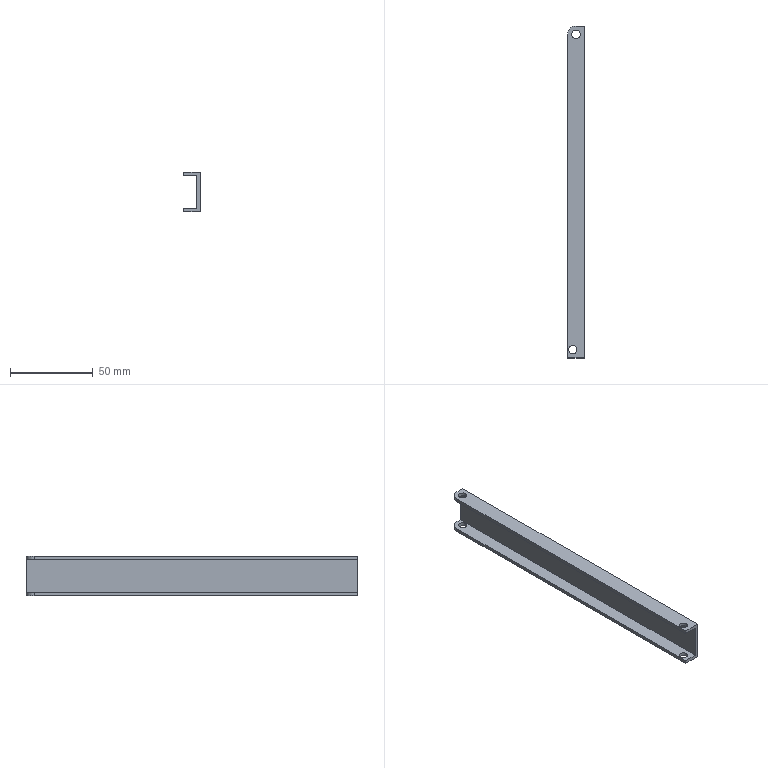Part | SolidWorks | features Cut 2, Extrusion 1, Fillet 1 | 1 solid | 20 faces | box 10 x 200 x 24 mm | volume 15821 mm3 | cylinder 10 | plane 10 | commonest cylinder face diameters 5 x8 10 x2
STEP:
#1=CARTESIAN_POINT('',(29.5,245.,0.));
#2=VERTEX_POINT('',#1);
#3=CARTESIAN_POINT('',(34.5,245.,0.));
#4=VERTEX_POINT('',#3);
#5=CARTESIAN_POINT('',(32.,245.,0.));
#6=DIRECTION('',(0.,0.,1.));
#7=DIRECTION('',(1.,0.,0.));
#8=AXIS2_PLACEMENT_3D('',#5,#6,#7);
#9=CIRCLE('',#8,2.5);
#10=EDGE_CURVE('',#2,#4,#9,.T.);
#11=ORIENTED_EDGE('',*,*,#10,.F.);
#12=CARTESIAN_POINT('',(29.5,245.,2.));
#13=VERTEX_POINT('',#12);
#14=CARTESIAN_POINT('',(29.5,245.,-22.));
#15=DIRECTION('',(0.,0.,1.));
#16=VECTOR('',#15,1000.);
#17=LINE('',#14,#16);
#18=EDGE_CURVE('',#2,#13,#17,.T.);
#19=ORIENTED_EDGE('',*,*,#18,.T.);
#20=CARTESIAN_POINT('',(34.5,245.,2.));
#21=VERTEX_POINT('',#20);
#22=CARTESIAN_POINT('',(32.,245.,2.));
#23=DIRECTION('',(0.,0.,1.));
#24=DIRECTION('',(1.,0.,0.));
#25=AXIS2_PLACEMENT_3D('',#22,#23,#24);
#26=CIRCLE('',#25,2.5);
#27=EDGE_CURVE('',#13,#21,#26,.T.);
#28=ORIENTED_EDGE('',*,*,#27,.T.);
#29=CARTESIAN_POINT('',(34.5,245.,-22.));
#30=DIRECTION('',(0.,0.,1.));
#31=VECTOR('',#30,1000.);
#32=LINE('',#29,#31);
#33=EDGE_CURVE('',#4,#21,#32,.T.);
#34=ORIENTED_EDGE('',*,*,#33,.F.);
#35=EDGE_LOOP('',(#11,#19,#28,#34));
#36=FACE_OUTER_BOUND('',#35,.T.);
#37=CARTESIAN_POINT('',(32.,245.,-22.));
#38=DIRECTION('',(0.,0.,1.));
#39=DIRECTION('',(1.,0.,0.));
#40=AXIS2_PLACEMENT_3D('',#37,#38,#39);
#41=CYLINDRICAL_SURFACE('',#40,2.5);
#42=ADVANCED_FACE('',(#36),#41,.F.);
#43=CARTESIAN_POINT('',(29.5,245.,-22.));
#44=VERTEX_POINT('',#43);
#45=CARTESIAN_POINT('',(34.5,245.,-22.));
#46=VERTEX_POINT('',#45);
#47=CARTESIAN_POINT('',(32.,245.,-22.));
#48=DIRECTION('',(0.,0.,1.));
#49=DIRECTION('',(1.,0.,0.));
#50=AXIS2_PLACEMENT_3D('',#47,#48,#49);
#51=CIRCLE('',#50,2.5);
#52=EDGE_CURVE('',#44,#46,#51,.T.);
#53=ORIENTED_EDGE('',*,*,#52,.F.);
#54=CARTESIAN_POINT('',(29.5,245.,-20.));
#55=VERTEX_POINT('',#54);
#56=CARTESIAN_POINT('',(29.5,245.,-22.));
#57=DIRECTION('',(0.,0.,1.));
#58=VECTOR('',#57,1000.);
#59=LINE('',#56,#58);
#60=EDGE_CURVE('',#44,#55,#59,.T.);
#61=ORIENTED_EDGE('',*,*,#60,.T.);
#62=CARTESIAN_POINT('',(34.5,245.,-20.));
#63=VERTEX_POINT('',#62);
#64=CARTESIAN_POINT('',(32.,245.,-20.));
#65=DIRECTION('',(0.,0.,-1.));
#66=DIRECTION('',(-1.,0.,0.));
#67=AXIS2_PLACEMENT_3D('',#64,#65,#66);
#68=CIRCLE('',#67,2.5);
#69=EDGE_CURVE('',#63,#55,#68,.T.);
#70=ORIENTED_EDGE('',*,*,#69,.F.);
#71=CARTESIAN_POINT('',(34.5,245.,-22.));
#72=DIRECTION('',(0.,0.,1.));
#73=VECTOR('',#72,1000.);
#74=LINE('',#71,#73);
#75=EDGE_CURVE('',#46,#63,#74,.T.);
#76=ORIENTED_EDGE('',*,*,#75,.F.);
#77=EDGE_LOOP('',(#53,#61,#70,#76));
#78=FACE_OUTER_BOUND('',#77,.T.);
#79=CARTESIAN_POINT('',(32.,245.,-22.));
#80=DIRECTION('',(0.,0.,1.));
#81=DIRECTION('',(1.,0.,0.));
#82=AXIS2_PLACEMENT_3D('',#79,#80,#81);
#83=CYLINDRICAL_SURFACE('',#82,2.5);
#84=ADVANCED_FACE('',(#78),#83,.F.);
#85=CARTESIAN_POINT('',(27.5,55.,0.));
#86=VERTEX_POINT('',#85);
#87=CARTESIAN_POINT('',(32.5,55.,0.));
#88=VERTEX_POINT('',#87);
#89=CARTESIAN_POINT('',(30.,55.,0.));
#90=DIRECTION('',(0.,0.,1.));
#91=DIRECTION('',(1.,0.,0.));
#92=AXIS2_PLACEMENT_3D('',#89,#90,#91);
#93=CIRCLE('',#92,2.5);
#94=EDGE_CURVE('',#86,#88,#93,.T.);
#95=ORIENTED_EDGE('',*,*,#94,.F.);
#96=CARTESIAN_POINT('',(27.5,55.,2.));
#97=VERTEX_POINT('',#96);
#98=CARTESIAN_POINT('',(27.5,55.,-22.));
#99=DIRECTION('',(0.,0.,1.));
#100=VECTOR('',#99,1000.);
#101=LINE('',#98,#100);
#102=EDGE_CURVE('',#86,#97,#101,.T.);
#103=ORIENTED_EDGE('',*,*,#102,.T.);
#104=CARTESIAN_POINT('',(32.5,55.,2.));
#105=VERTEX_POINT('',#104);
#106=CARTESIAN_POINT('',(30.,55.,2.));
#107=DIRECTION('',(0.,0.,-1.));
#108=DIRECTION('',(-1.,0.,0.));
#109=AXIS2_PLACEMENT_3D('',#106,#107,#108);
#110=CIRCLE('',#109,2.5);
#111=EDGE_CURVE('',#105,#97,#110,.T.);
#112=ORIENTED_EDGE('',*,*,#111,.F.);
#113=CARTESIAN_POINT('',(32.5,55.,-22.));
#114=DIRECTION('',(0.,0.,1.));
#115=VECTOR('',#114,1000.);
#116=LINE('',#113,#115);
#117=EDGE_CURVE('',#88,#105,#116,.T.);
#118=ORIENTED_EDGE('',*,*,#117,.F.);
#119=EDGE_LOOP('',(#95,#103,#112,#118));
#120=FACE_OUTER_BOUND('',#119,.T.);
#121=CARTESIAN_POINT('',(30.,55.,-22.));
#122=DIRECTION('',(0.,0.,1.));
#123=DIRECTION('',(1.,0.,0.));
#124=AXIS2_PLACEMENT_3D('',#121,#122,#123);
#125=CYLINDRICAL_SURFACE('',#124,2.5);
#126=ADVANCED_FACE('',(#120),#125,.F.);
#127=CARTESIAN_POINT('',(27.5,55.,-22.));
#128=VERTEX_POINT('',#127);
#129=CARTESIAN_POINT('',(32.5,55.,-22.));
#130=VERTEX_POINT('',#129);
#131=CARTESIAN_POINT('',(30.,55.,-22.));
#132=DIRECTION('',(0.,0.,1.));
#133=DIRECTION('',(1.,0.,0.));
#134=AXIS2_PLACEMENT_3D('',#131,#132,#133);
#135=CIRCLE('',#134,2.5);
#136=EDGE_CURVE('',#128,#130,#135,.T.);
#137=ORIENTED_EDGE('',*,*,#136,.F.);
#138=CARTESIAN_POINT('',(27.5,55.,-20.));
#139=VERTEX_POINT('',#138);
#140=CARTESIAN_POINT('',(27.5,55.,-22.));
#141=DIRECTION('',(0.,0.,1.));
#142=VECTOR('',#141,1000.);
#143=LINE('',#140,#142);
#144=EDGE_CURVE('',#128,#139,#143,.T.);
#145=ORIENTED_EDGE('',*,*,#144,.T.);
#146=CARTESIAN_POINT('',(32.5,55.,-20.));
#147=VERTEX_POINT('',#146);
#148=CARTESIAN_POINT('',(30.,55.,-20.));
#149=DIRECTION('',(0.,0.,-1.));
#150=DIRECTION('',(-1.,0.,0.));
#151=AXIS2_PLACEMENT_3D('',#148,#149,#150);
#152=CIRCLE('',#151,2.5);
#153=EDGE_CURVE('',#147,#139,#152,.T.);
#154=ORIENTED_EDGE('',*,*,#153,.F.);
#155=CARTESIAN_POINT('',(32.5,55.,-22.));
#156=DIRECTION('',(0.,0.,1.));
#157=VECTOR('',#156,1000.);
#158=LINE('',#155,#157);
#159=EDGE_CURVE('',#130,#147,#158,.T.);
#160=ORIENTED_EDGE('',*,*,#159,.F.);
#161=EDGE_LOOP('',(#137,#145,#154,#160));
#162=FACE_OUTER_BOUND('',#161,.T.);
#163=CARTESIAN_POINT('',(30.,55.,-22.));
#164=DIRECTION('',(0.,0.,1.));
#165=DIRECTION('',(1.,0.,0.));
#166=AXIS2_PLACEMENT_3D('',#163,#164,#165);
#167=CYLINDRICAL_SURFACE('',#166,2.5);
#168=ADVANCED_FACE('',(#162),#167,.F.);
#169=CARTESIAN_POINT('',(32.,245.,0.));
#170=DIRECTION('',(0.,0.,1.));
#171=DIRECTION('',(1.,0.,0.));
#172=AXIS2_PLACEMENT_3D('',#169,#170,#171);
#173=CIRCLE('',#172,2.5);
#174=EDGE_CURVE('',#4,#2,#173,.T.);
#175=ORIENTED_EDGE('',*,*,#174,.T.);
#176=ORIENTED_EDGE('',*,*,#10,.T.);
#177=EDGE_LOOP('',(#175,#176));
#178=FACE_BOUND('',#177,.T.);
#179=CARTESIAN_POINT('',(30.,55.,0.));
#180=DIRECTION('',(0.,0.,1.));
#181=DIRECTION('',(1.,0.,0.));
#182=AXIS2_PLACEMENT_3D('',#179,#180,#181);
#183=CIRCLE('',#182,2.5);
#184=EDGE_CURVE('',#88,#86,#183,.T.);
#185=ORIENTED_EDGE('',*,*,#184,.T.);
#186=ORIENTED_EDGE('',*,*,#94,.T.);
#187=EDGE_LOOP('',(#185,#186));
#188=FACE_BOUND('',#187,.T.);
#189=CARTESIAN_POINT('',(27.,245.,0.));
#190=VERTEX_POINT('',#189);
#191=CARTESIAN_POINT('',(27.,50.,0.));
#192=VERTEX_POINT('',#191);
#193=CARTESIAN_POINT('',(27.,250.,0.));
#194=DIRECTION('',(0.,-1.,0.));
#195=VECTOR('',#194,1000.);
#196=LINE('',#193,#195);
#197=EDGE_CURVE('',#190,#192,#196,.T.);
#198=ORIENTED_EDGE('',*,*,#197,.F.);
#199=CARTESIAN_POINT('',(32.,250.,0.));
#200=VERTEX_POINT('',#199);
#201=CARTESIAN_POINT('',(32.,245.,0.));
#202=DIRECTION('',(0.,0.,-1.));
#203=DIRECTION('',(1.,0.,0.));
#204=AXIS2_PLACEMENT_3D('',#201,#202,#203);
#205=CIRCLE('',#204,5.);
#206=EDGE_CURVE('',#190,#200,#205,.T.);
#207=ORIENTED_EDGE('',*,*,#206,.T.);
#208=CARTESIAN_POINT('',(35.,250.,0.));
#209=VERTEX_POINT('',#208);
#210=CARTESIAN_POINT('',(27.,250.,0.));
#211=DIRECTION('',(-1.,0.,0.));
#212=VECTOR('',#211,1000.);
#213=LINE('',#210,#212);
#214=EDGE_CURVE('',#209,#200,#213,.T.);
#215=ORIENTED_EDGE('',*,*,#214,.F.);
#216=CARTESIAN_POINT('',(35.,50.,0.));
#217=VERTEX_POINT('',#216);
#218=CARTESIAN_POINT('',(35.,250.,0.));
#219=DIRECTION('',(0.,-1.,0.));
#220=VECTOR('',#219,1000.);
#221=LINE('',#218,#220);
#222=EDGE_CURVE('',#209,#217,#221,.T.);
#223=ORIENTED_EDGE('',*,*,#222,.T.);
#224=CARTESIAN_POINT('',(27.,50.,0.));
#225=DIRECTION('',(-1.,0.,0.));
#226=VECTOR('',#225,1000.);
#227=LINE('',#224,#226);
#228=EDGE_CURVE('',#217,#192,#227,.T.);
#229=ORIENTED_EDGE('',*,*,#228,.T.);
#230=EDGE_LOOP('',(#198,#207,#215,#223,#229));
#231=FACE_OUTER_BOUND('',#230,.T.);
#232=CARTESIAN_POINT('',(27.,250.,0.));
#233=DIRECTION('',(0.,0.,1.));
#234=DIRECTION('',(1.,0.,0.));
#235=AXIS2_PLACEMENT_3D('',#232,#233,#234);
#236=PLANE('',#235);
#237=ADVANCED_FACE('',(#178,#188,#231),#236,.F.);
#238=CARTESIAN_POINT('',(27.,245.,2.));
#239=VERTEX_POINT('',#238);
#240=CARTESIAN_POINT('',(27.,50.,2.));
#241=VERTEX_POINT('',#240);
#242=CARTESIAN_POINT('',(27.,250.,2.));
#243=DIRECTION('',(0.,-1.,0.));
#244=VECTOR('',#243,1000.);
#245=LINE('',#242,#244);
#246=EDGE_CURVE('',#239,#241,#245,.T.);
#247=ORIENTED_EDGE('',*,*,#246,.F.);
#248=CARTESIAN_POINT('',(27.,245.,0.));
#249=DIRECTION('',(0.,0.,-1.));
#250=VECTOR('',#249,1000.);
#251=LINE('',#248,#250);
#252=EDGE_CURVE('',#239,#190,#251,.T.);
#253=ORIENTED_EDGE('',*,*,#252,.T.);
#254=ORIENTED_EDGE('',*,*,#197,.T.);
#255=CARTESIAN_POINT('',(27.,50.,2.));
#256=DIRECTION('',(0.,0.,1.));
#257=VECTOR('',#256,1000.);
#258=LINE('',#255,#257);
#259=EDGE_CURVE('',#192,#241,#258,.T.);
#260=ORIENTED_EDGE('',*,*,#259,.T.);
#261=EDGE_LOOP('',(#247,#253,#254,#260));
#262=FACE_OUTER_BOUND('',#261,.T.);
#263=CARTESIAN_POINT('',(27.,250.,2.));
#264=DIRECTION('',(1.,0.,0.));
#265=DIRECTION('',(0.,0.,-1.));
#266=AXIS2_PLACEMENT_3D('',#263,#264,#265);
#267=PLANE('',#266);
#268=ADVANCED_FACE('',(#262),#267,.F.);
#269=CARTESIAN_POINT('',(32.,245.,2.));
#270=DIRECTION('',(0.,0.,1.));
#271=DIRECTION('',(1.,0.,0.));
#272=AXIS2_PLACEMENT_3D('',#269,#270,#271);
#273=CIRCLE('',#272,2.5);
#274=EDGE_CURVE('',#21,#13,#273,.T.);
#275=ORIENTED_EDGE('',*,*,#274,.F.);
#276=ORIENTED_EDGE('',*,*,#27,.F.);
#277=EDGE_LOOP('',(#275,#276));
#278=FACE_BOUND('',#277,.T.);
#279=ORIENTED_EDGE('',*,*,#111,.T.);
#280=CARTESIAN_POINT('',(30.,55.,2.));
#281=DIRECTION('',(0.,0.,-1.));
#282=DIRECTION('',(-1.,0.,0.));
#283=AXIS2_PLACEMENT_3D('',#280,#281,#282);
#284=CIRCLE('',#283,2.5);
#285=EDGE_CURVE('',#97,#105,#284,.T.);
#286=ORIENTED_EDGE('',*,*,#285,.T.);
#287=EDGE_LOOP('',(#279,#286));
#288=FACE_BOUND('',#287,.T.);
#289=CARTESIAN_POINT('',(32.,250.,2.));
#290=VERTEX_POINT('',#289);
#291=CARTESIAN_POINT('',(37.,250.,2.));
#292=VERTEX_POINT('',#291);
#293=CARTESIAN_POINT('',(37.,250.,2.));
#294=DIRECTION('',(1.,0.,0.));
#295=VECTOR('',#294,1000.);
#296=LINE('',#293,#295);
#297=EDGE_CURVE('',#290,#292,#296,.T.);
#298=ORIENTED_EDGE('',*,*,#297,.F.);
#299=CARTESIAN_POINT('',(32.,245.,2.));
#300=DIRECTION('',(0.,0.,1.));
#301=DIRECTION('',(-1.,0.,0.));
#302=AXIS2_PLACEMENT_3D('',#299,#300,#301);
#303=CIRCLE('',#302,5.);
#304=EDGE_CURVE('',#290,#239,#303,.T.);
#305=ORIENTED_EDGE('',*,*,#304,.T.);
#306=ORIENTED_EDGE('',*,*,#246,.T.);
#307=CARTESIAN_POINT('',(37.,50.,2.));
#308=VERTEX_POINT('',#307);
#309=CARTESIAN_POINT('',(37.,50.,2.));
#310=DIRECTION('',(1.,0.,0.));
#311=VECTOR('',#310,1000.);
#312=LINE('',#309,#311);
#313=EDGE_CURVE('',#241,#308,#312,.T.);
#314=ORIENTED_EDGE('',*,*,#313,.T.);
#315=CARTESIAN_POINT('',(37.,250.,2.));
#316=DIRECTION('',(0.,-1.,0.));
#317=VECTOR('',#316,1000.);
#318=LINE('',#315,#317);
#319=EDGE_CURVE('',#292,#308,#318,.T.);
#320=ORIENTED_EDGE('',*,*,#319,.F.);
#321=EDGE_LOOP('',(#298,#305,#306,#314,#320));
#322=FACE_OUTER_BOUND('',#321,.T.);
#323=CARTESIAN_POINT('',(37.,250.,2.));
#324=DIRECTION('',(0.,0.,-1.));
#325=DIRECTION('',(-1.,0.,0.));
#326=AXIS2_PLACEMENT_3D('',#323,#324,#325);
#327=PLANE('',#326);
#328=ADVANCED_FACE('',(#278,#288,#322),#327,.F.);
#329=CARTESIAN_POINT('',(37.,50.,-22.));
#330=VERTEX_POINT('',#329);
#331=CARTESIAN_POINT('',(37.,50.,-22.));
#332=DIRECTION('',(0.,0.,-1.));
#333=VECTOR('',#332,1000.);
#334=LINE('',#331,#333);
#335=EDGE_CURVE('',#308,#330,#334,.T.);
#336=ORIENTED_EDGE('',*,*,#335,.T.);
#337=CARTESIAN_POINT('',(37.,250.,-22.));
#338=VERTEX_POINT('',#337);
#339=CARTESIAN_POINT('',(37.,250.,-22.));
#340=DIRECTION('',(0.,-1.,0.));
#341=VECTOR('',#340,1000.);
#342=LINE('',#339,#341);
#343=EDGE_CURVE('',#338,#330,#342,.T.);
#344=ORIENTED_EDGE('',*,*,#343,.F.);
#345=CARTESIAN_POINT('',(37.,250.,-22.));
#346=DIRECTION('',(0.,0.,-1.));
#347=VECTOR('',#346,1000.);
#348=LINE('',#345,#347);
#349=EDGE_CURVE('',#292,#338,#348,.T.);
#350=ORIENTED_EDGE('',*,*,#349,.F.);
#351=ORIENTED_EDGE('',*,*,#319,.T.);
#352=EDGE_LOOP('',(#336,#344,#350,#351));
#353=FACE_OUTER_BOUND('',#352,.T.);
#354=CARTESIAN_POINT('',(37.,250.,-22.));
#355=DIRECTION('',(-1.,0.,0.));
#356=DIRECTION('',(0.,0.,1.));
#357=AXIS2_PLACEMENT_3D('',#354,#355,#356);
#358=PLANE('',#357);
#359=ADVANCED_FACE('',(#353),#358,.F.);
#360=CARTESIAN_POINT('',(32.,245.,-22.));
#361=DIRECTION('',(0.,0.,1.));
#362=DIRECTION('',(1.,0.,0.));
#363=AXIS2_PLACEMENT_3D('',#360,#361,#362);
#364=CIRCLE('',#363,2.5);
#365=EDGE_CURVE('',#46,#44,#364,.T.);
#366=ORIENTED_EDGE('',*,*,#365,.T.);
#367=ORIENTED_EDGE('',*,*,#52,.T.);
#368=EDGE_LOOP('',(#366,#367));
#369=FACE_BOUND('',#368,.T.);
#370=CARTESIAN_POINT('',(30.,55.,-22.));
#371=DIRECTION('',(0.,0.,1.));
#372=DIRECTION('',(1.,0.,0.));
#373=AXIS2_PLACEMENT_3D('',#370,#371,#372);
#374=CIRCLE('',#373,2.5);
#375=EDGE_CURVE('',#130,#128,#374,.T.);
#376=ORIENTED_EDGE('',*,*,#375,.T.);
#377=ORIENTED_EDGE('',*,*,#136,.T.);
#378=EDGE_LOOP('',(#376,#377));
#379=FACE_BOUND('',#378,.T.);
#380=CARTESIAN_POINT('',(27.,245.,-22.));
#381=VERTEX_POINT('',#380);
#382=CARTESIAN_POINT('',(27.,50.,-22.));
#383=VERTEX_POINT('',#382);
#384=CARTESIAN_POINT('',(27.,250.,-22.));
#385=DIRECTION('',(0.,-1.,0.));
#386=VECTOR('',#385,1000.);
#387=LINE('',#384,#386);
#388=EDGE_CURVE('',#381,#383,#387,.T.);
#389=ORIENTED_EDGE('',*,*,#388,.F.);
#390=CARTESIAN_POINT('',(32.,250.,-22.));
#391=VERTEX_POINT('',#390);
#392=CARTESIAN_POINT('',(32.,245.,-22.));
#393=DIRECTION('',(0.,0.,-1.));
#394=DIRECTION('',(1.,0.,0.));
#395=AXIS2_PLACEMENT_3D('',#392,#393,#394);
#396=CIRCLE('',#395,5.);
#397=EDGE_CURVE('',#381,#391,#396,.T.);
#398=ORIENTED_EDGE('',*,*,#397,.T.);
#399=CARTESIAN_POINT('',(27.,250.,-22.));
#400=DIRECTION('',(-1.,0.,0.));
#401=VECTOR('',#400,1000.);
#402=LINE('',#399,#401);
#403=EDGE_CURVE('',#338,#391,#402,.T.);
#404=ORIENTED_EDGE('',*,*,#403,.F.);
#405=ORIENTED_EDGE('',*,*,#343,.T.);
#406=CARTESIAN_POINT('',(27.,50.,-22.));
#407=DIRECTION('',(-1.,0.,0.));
#408=VECTOR('',#407,1000.);
#409=LINE('',#406,#408);
#410=EDGE_CURVE('',#330,#383,#409,.T.);
#411=ORIENTED_EDGE('',*,*,#410,.T.);
#412=EDGE_LOOP('',(#389,#398,#404,#405,#411));
#413=FACE_OUTER_BOUND('',#412,.T.);
#414=CARTESIAN_POINT('',(27.,250.,-22.));
#415=DIRECTION('',(0.,0.,1.));
#416=DIRECTION('',(1.,0.,0.));
#417=AXIS2_PLACEMENT_3D('',#414,#415,#416);
#418=PLANE('',#417);
#419=ADVANCED_FACE('',(#369,#379,#413),#418,.F.);
#420=CARTESIAN_POINT('',(27.,245.,-20.));
#421=VERTEX_POINT('',#420);
#422=CARTESIAN_POINT('',(27.,50.,-20.));
#423=VERTEX_POINT('',#422);
#424=CARTESIAN_POINT('',(27.,250.,-20.));
#425=DIRECTION('',(0.,-1.,0.));
#426=VECTOR('',#425,1000.);
#427=LINE('',#424,#426);
#428=EDGE_CURVE('',#421,#423,#427,.T.);
#429=ORIENTED_EDGE('',*,*,#428,.F.);
#430=CARTESIAN_POINT('',(27.,245.,-22.));
#431=DIRECTION('',(0.,0.,-1.));
#432=VECTOR('',#431,1000.);
#433=LINE('',#430,#432);
#434=EDGE_CURVE('',#421,#381,#433,.T.);
#435=ORIENTED_EDGE('',*,*,#434,.T.);
#436=ORIENTED_EDGE('',*,*,#388,.T.);
#437=CARTESIAN_POINT('',(27.,50.,-20.));
#438=DIRECTION('',(0.,0.,1.));
#439=VECTOR('',#438,1000.);
#440=LINE('',#437,#439);
#441=EDGE_CURVE('',#383,#423,#440,.T.);
#442=ORIENTED_EDGE('',*,*,#441,.T.);
#443=EDGE_LOOP('',(#429,#435,#436,#442));
#444=FACE_OUTER_BOUND('',#443,.T.);
#445=CARTESIAN_POINT('',(27.,250.,-20.));
#446=DIRECTION('',(1.,0.,0.));
#447=DIRECTION('',(0.,0.,-1.));
#448=AXIS2_PLACEMENT_3D('',#445,#446,#447);
#449=PLANE('',#448);
#450=ADVANCED_FACE('',(#444),#449,.F.);
#451=ORIENTED_EDGE('',*,*,#69,.T.);
#452=CARTESIAN_POINT('',(32.,245.,-20.));
#453=DIRECTION('',(0.,0.,-1.));
#454=DIRECTION('',(-1.,0.,0.));
#455=AXIS2_PLACEMENT_3D('',#452,#453,#454);
#456=CIRCLE('',#455,2.5);
#457=EDGE_CURVE('',#55,#63,#456,.T.);
#458=ORIENTED_EDGE('',*,*,#457,.T.);
#459=EDGE_LOOP('',(#451,#458));
#460=FACE_BOUND('',#459,.T.);
#461=ORIENTED_EDGE('',*,*,#153,.T.);
#462=CARTESIAN_POINT('',(30.,55.,-20.));
#463=DIRECTION('',(0.,0.,-1.));
#464=DIRECTION('',(-1.,0.,0.));
#465=AXIS2_PLACEMENT_3D('',#462,#463,#464);
#466=CIRCLE('',#465,2.5);
#467=EDGE_CURVE('',#139,#147,#466,.T.);
#468=ORIENTED_EDGE('',*,*,#467,.T.);
#469=EDGE_LOOP('',(#461,#468));
#470=FACE_BOUND('',#469,.T.);
#471=CARTESIAN_POINT('',(32.,250.,-20.));
#472=VERTEX_POINT('',#471);
#473=CARTESIAN_POINT('',(35.,250.,-20.));
#474=VERTEX_POINT('',#473);
#475=CARTESIAN_POINT('',(35.,250.,-20.));
#476=DIRECTION('',(1.,0.,0.));
#477=VECTOR('',#476,1000.);
#478=LINE('',#475,#477);
#479=EDGE_CURVE('',#472,#474,#478,.T.);
#480=ORIENTED_EDGE('',*,*,#479,.F.);
#481=CARTESIAN_POINT('',(32.,245.,-20.));
#482=DIRECTION('',(0.,0.,1.));
#483=DIRECTION('',(-1.,0.,0.));
#484=AXIS2_PLACEMENT_3D('',#481,#482,#483);
#485=CIRCLE('',#484,5.);
#486=EDGE_CURVE('',#472,#421,#485,.T.);
#487=ORIENTED_EDGE('',*,*,#486,.T.);
#488=ORIENTED_EDGE('',*,*,#428,.T.);
#489=CARTESIAN_POINT('',(35.,50.,-20.));
#490=VERTEX_POINT('',#489);
#491=CARTESIAN_POINT('',(35.,50.,-20.));
#492=DIRECTION('',(1.,0.,0.));
#493=VECTOR('',#492,1000.);
#494=LINE('',#491,#493);
#495=EDGE_CURVE('',#423,#490,#494,.T.);
#496=ORIENTED_EDGE('',*,*,#495,.T.);
#497=CARTESIAN_POINT('',(35.,250.,-20.));
#498=DIRECTION('',(0.,-1.,0.));
#499=VECTOR('',#498,1000.);
#500=LINE('',#497,#499);
#501=EDGE_CURVE('',#474,#490,#500,.T.);
#502=ORIENTED_EDGE('',*,*,#501,.F.);
#503=EDGE_LOOP('',(#480,#487,#488,#496,#502));
#504=FACE_OUTER_BOUND('',#503,.T.);
#505=CARTESIAN_POINT('',(35.,250.,-20.));
#506=DIRECTION('',(0.,0.,-1.));
#507=DIRECTION('',(-1.,0.,0.));
#508=AXIS2_PLACEMENT_3D('',#505,#506,#507);
#509=PLANE('',#508);
#510=ADVANCED_FACE('',(#460,#470,#504),#509,.F.);
#511=CARTESIAN_POINT('',(35.,50.,-10.));
#512=DIRECTION('',(0.,0.,1.));
#513=VECTOR('',#512,1000.);
#514=LINE('',#511,#513);
#515=EDGE_CURVE('',#490,#217,#514,.T.);
#516=ORIENTED_EDGE('',*,*,#515,.T.);
#517=ORIENTED_EDGE('',*,*,#222,.F.);
#518=CARTESIAN_POINT('',(35.,250.,0.));
#519=DIRECTION('',(0.,0.,1.));
#520=VECTOR('',#519,1000.);
#521=LINE('',#518,#520);
#522=EDGE_CURVE('',#474,#209,#521,.T.);
#523=ORIENTED_EDGE('',*,*,#522,.F.);
#524=ORIENTED_EDGE('',*,*,#501,.T.);
#525=EDGE_LOOP('',(#516,#517,#523,#524));
#526=FACE_OUTER_BOUND('',#525,.T.);
#527=CARTESIAN_POINT('',(35.,250.,-10.));
#528=DIRECTION('',(1.,0.,0.));
#529=DIRECTION('',(0.,0.,-1.));
#530=AXIS2_PLACEMENT_3D('',#527,#528,#529);
#531=PLANE('',#530);
#532=ADVANCED_FACE('',(#526),#531,.F.);
#533=ORIENTED_EDGE('',*,*,#403,.T.);
#534=CARTESIAN_POINT('',(32.,250.,-20.));
#535=DIRECTION('',(0.,0.,1.));
#536=VECTOR('',#535,1000.);
#537=LINE('',#534,#536);
#538=EDGE_CURVE('',#391,#472,#537,.T.);
#539=ORIENTED_EDGE('',*,*,#538,.T.);
#540=ORIENTED_EDGE('',*,*,#479,.T.);
#541=ORIENTED_EDGE('',*,*,#522,.T.);
#542=ORIENTED_EDGE('',*,*,#214,.T.);
#543=CARTESIAN_POINT('',(32.,250.,2.));
#544=DIRECTION('',(0.,0.,1.));
#545=VECTOR('',#544,1000.);
#546=LINE('',#543,#545);
#547=EDGE_CURVE('',#200,#290,#546,.T.);
#548=ORIENTED_EDGE('',*,*,#547,.T.);
#549=ORIENTED_EDGE('',*,*,#297,.T.);
#550=ORIENTED_EDGE('',*,*,#349,.T.);
#551=EDGE_LOOP('',(#533,#539,#540,#541,#542,#548,#549,#550));
#552=FACE_OUTER_BOUND('',#551,.T.);
#553=CARTESIAN_POINT('',(0.,250.,0.));
#554=DIRECTION('',(0.,1.,0.));
#555=DIRECTION('',(0.,0.,1.));
#556=AXIS2_PLACEMENT_3D('',#553,#554,#555);
#557=PLANE('',#556);
#558=ADVANCED_FACE('',(#552),#557,.T.);
#559=ORIENTED_EDGE('',*,*,#228,.F.);
#560=ORIENTED_EDGE('',*,*,#515,.F.);
#561=ORIENTED_EDGE('',*,*,#495,.F.);
#562=ORIENTED_EDGE('',*,*,#441,.F.);
#563=ORIENTED_EDGE('',*,*,#410,.F.);
#564=ORIENTED_EDGE('',*,*,#335,.F.);
#565=ORIENTED_EDGE('',*,*,#313,.F.);
#566=ORIENTED_EDGE('',*,*,#259,.F.);
#567=EDGE_LOOP('',(#559,#560,#561,#562,#563,#564,#565,#566));
#568=FACE_OUTER_BOUND('',#567,.T.);
#569=CARTESIAN_POINT('',(0.,50.,0.));
#570=DIRECTION('',(0.,1.,0.));
#571=DIRECTION('',(0.,0.,1.));
#572=AXIS2_PLACEMENT_3D('',#569,#570,#571);
#573=PLANE('',#572);
#574=ADVANCED_FACE('',(#568),#573,.F.);
#575=ORIENTED_EDGE('',*,*,#144,.F.);
#576=ORIENTED_EDGE('',*,*,#375,.F.);
#577=ORIENTED_EDGE('',*,*,#159,.T.);
#578=ORIENTED_EDGE('',*,*,#467,.F.);
#579=EDGE_LOOP('',(#575,#576,#577,#578));
#580=FACE_OUTER_BOUND('',#579,.T.);
#581=CARTESIAN_POINT('',(30.,55.,-22.));
#582=DIRECTION('',(0.,0.,1.));
#583=DIRECTION('',(1.,0.,0.));
#584=AXIS2_PLACEMENT_3D('',#581,#582,#583);
#585=CYLINDRICAL_SURFACE('',#584,2.5);
#586=ADVANCED_FACE('',(#580),#585,.F.);
#587=ORIENTED_EDGE('',*,*,#102,.F.);
#588=ORIENTED_EDGE('',*,*,#184,.F.);
#589=ORIENTED_EDGE('',*,*,#117,.T.);
#590=ORIENTED_EDGE('',*,*,#285,.F.);
#591=EDGE_LOOP('',(#587,#588,#589,#590));
#592=FACE_OUTER_BOUND('',#591,.T.);
#593=CARTESIAN_POINT('',(30.,55.,-22.));
#594=DIRECTION('',(0.,0.,1.));
#595=DIRECTION('',(1.,0.,0.));
#596=AXIS2_PLACEMENT_3D('',#593,#594,#595);
#597=CYLINDRICAL_SURFACE('',#596,2.5);
#598=ADVANCED_FACE('',(#592),#597,.F.);
#599=ORIENTED_EDGE('',*,*,#397,.F.);
#600=ORIENTED_EDGE('',*,*,#434,.F.);
#601=ORIENTED_EDGE('',*,*,#486,.F.);
#602=ORIENTED_EDGE('',*,*,#538,.F.);
#603=EDGE_LOOP('',(#599,#600,#601,#602));
#604=FACE_OUTER_BOUND('',#603,.T.);
#605=CARTESIAN_POINT('',(32.,245.,0.));
#606=DIRECTION('',(0.,0.,-1.));
#607=DIRECTION('',(-1.,0.,0.));
#608=AXIS2_PLACEMENT_3D('',#605,#606,#607);
#609=CYLINDRICAL_SURFACE('',#608,5.);
#610=ADVANCED_FACE('',(#604),#609,.T.);
#611=ORIENTED_EDGE('',*,*,#206,.F.);
#612=ORIENTED_EDGE('',*,*,#252,.F.);
#613=ORIENTED_EDGE('',*,*,#304,.F.);
#614=ORIENTED_EDGE('',*,*,#547,.F.);
#615=EDGE_LOOP('',(#611,#612,#613,#614));
#616=FACE_OUTER_BOUND('',#615,.T.);
#617=CARTESIAN_POINT('',(32.,245.,0.));
#618=DIRECTION('',(0.,0.,-1.));
#619=DIRECTION('',(-1.,0.,0.));
#620=AXIS2_PLACEMENT_3D('',#617,#618,#619);
#621=CYLINDRICAL_SURFACE('',#620,5.);
#622=ADVANCED_FACE('',(#616),#621,.T.);
#623=ORIENTED_EDGE('',*,*,#60,.F.);
#624=ORIENTED_EDGE('',*,*,#365,.F.);
#625=ORIENTED_EDGE('',*,*,#75,.T.);
#626=ORIENTED_EDGE('',*,*,#457,.F.);
#627=EDGE_LOOP('',(#623,#624,#625,#626));
#628=FACE_OUTER_BOUND('',#627,.T.);
#629=CARTESIAN_POINT('',(32.,245.,-22.));
#630=DIRECTION('',(0.,0.,1.));
#631=DIRECTION('',(1.,0.,0.));
#632=AXIS2_PLACEMENT_3D('',#629,#630,#631);
#633=CYLINDRICAL_SURFACE('',#632,2.5);
#634=ADVANCED_FACE('',(#628),#633,.F.);
#635=ORIENTED_EDGE('',*,*,#18,.F.);
#636=ORIENTED_EDGE('',*,*,#174,.F.);
#637=ORIENTED_EDGE('',*,*,#33,.T.);
#638=ORIENTED_EDGE('',*,*,#274,.T.);
#639=EDGE_LOOP('',(#635,#636,#637,#638));
#640=FACE_OUTER_BOUND('',#639,.T.);
#641=CARTESIAN_POINT('',(32.,245.,-22.));
#642=DIRECTION('',(0.,0.,1.));
#643=DIRECTION('',(1.,0.,0.));
#644=AXIS2_PLACEMENT_3D('',#641,#642,#643);
#645=CYLINDRICAL_SURFACE('',#644,2.5);
#646=ADVANCED_FACE('',(#640),#645,.F.);
#647=CLOSED_SHELL('',(#42,#84,#126,#168,#237,#268,#328,#359,#419,#450,#510,#532,#558,#574,#586,#598,#610,#622,#634,#646));
#648=MANIFOLD_SOLID_BREP('',#647);
#649=CARTESIAN_POINT('',(0.,0.,0.));
#650=DIRECTION('',(0.,0.,1.));
#651=DIRECTION('',(1.,0.,0.));
#652=AXIS2_PLACEMENT_3D('',#649,#650,#651);
#653=(LENGTH_UNIT()NAMED_UNIT(*)SI_UNIT(.MILLI.,.METRE.));
#654=UNCERTAINTY_MEASURE_WITH_UNIT(LENGTH_MEASURE(0.00001),#653,'','');
#655=(NAMED_UNIT(*)PLANE_ANGLE_UNIT()SI_UNIT($,.RADIAN.));
#656=(NAMED_UNIT(*)SI_UNIT($,.STERADIAN.)SOLID_ANGLE_UNIT());
#657=(GEOMETRIC_REPRESENTATION_CONTEXT(3)GLOBAL_UNCERTAINTY_ASSIGNED_CONTEXT((#654))GLOBAL_UNIT_ASSIGNED_CONTEXT((#653,#655,#656))REPRESENTATION_CONTEXT('',''));
#658=ADVANCED_BREP_SHAPE_REPRESENTATION('',(#648,#652),#657);